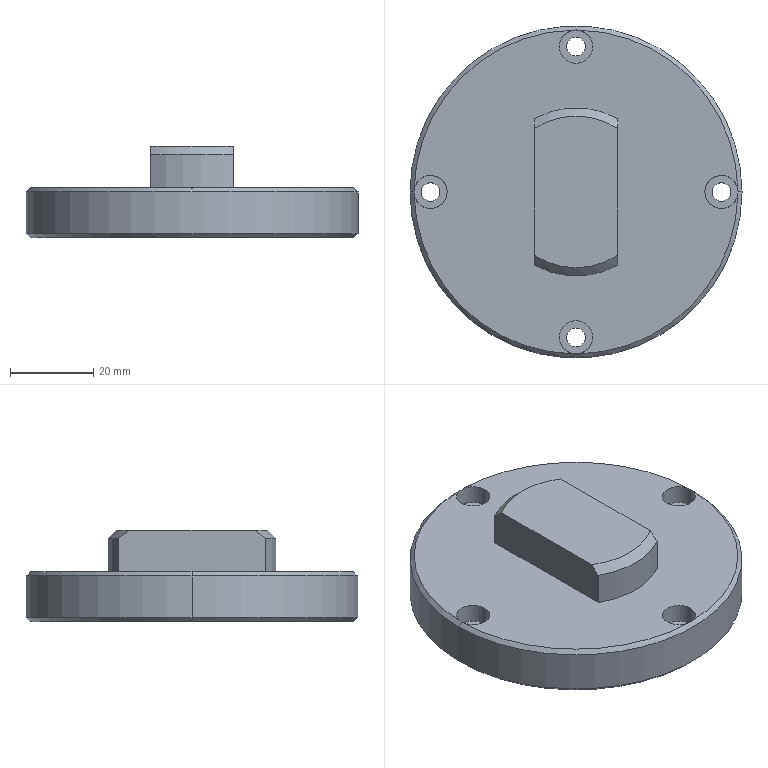Part | STEP file | TJ-DHQM-004-010 | 1 solid | 35 faces | box 79.9 x 79.9 x 22 mm | volume 66197 mm3 | cylinder 20 | plane 9 | cone 6 | commonest cylinder face diameters 4.5 x8 8 x8 40.5 x2 79.9 x2
STEP:
#1=CARTESIAN_POINT('',(-4.,35.,7.4));
#2=VERTEX_POINT('',#1);
#3=CARTESIAN_POINT('',(4.,35.,7.4));
#4=VERTEX_POINT('',#3);
#5=CARTESIAN_POINT('',(0.,35.,7.4));
#6=DIRECTION('',(0.,0.,1.));
#7=DIRECTION('',(1.,0.,0.));
#8=AXIS2_PLACEMENT_3D('',#5,#6,#7);
#9=CIRCLE('',#8,4.);
#10=EDGE_CURVE('',#2,#4,#9,.T.);
#11=ORIENTED_EDGE('',*,*,#10,.F.);
#12=CARTESIAN_POINT('',(-4.,35.,12.));
#13=VERTEX_POINT('',#12);
#14=CARTESIAN_POINT('',(-4.,35.,12.));
#15=DIRECTION('',(0.,0.,1.));
#16=VECTOR('',#15,1000.);
#17=LINE('',#14,#16);
#18=EDGE_CURVE('',#2,#13,#17,.T.);
#19=ORIENTED_EDGE('',*,*,#18,.T.);
#20=CARTESIAN_POINT('',(4.,35.,12.));
#21=VERTEX_POINT('',#20);
#22=CARTESIAN_POINT('',(0.,35.,12.));
#23=DIRECTION('',(0.,0.,1.));
#24=DIRECTION('',(1.,0.,0.));
#25=AXIS2_PLACEMENT_3D('',#22,#23,#24);
#26=CIRCLE('',#25,4.);
#27=EDGE_CURVE('',#13,#21,#26,.T.);
#28=ORIENTED_EDGE('',*,*,#27,.T.);
#29=CARTESIAN_POINT('',(4.,35.,12.));
#30=DIRECTION('',(0.,0.,1.));
#31=VECTOR('',#30,1000.);
#32=LINE('',#29,#31);
#33=EDGE_CURVE('',#4,#21,#32,.T.);
#34=ORIENTED_EDGE('',*,*,#33,.F.);
#35=EDGE_LOOP('',(#11,#19,#28,#34));
#36=FACE_OUTER_BOUND('',#35,.T.);
#37=CARTESIAN_POINT('',(0.,35.,12.));
#38=DIRECTION('',(0.,0.,1.));
#39=DIRECTION('',(1.,0.,0.));
#40=AXIS2_PLACEMENT_3D('',#37,#38,#39);
#41=CYLINDRICAL_SURFACE('',#40,4.);
#42=ADVANCED_FACE('',(#36),#41,.F.);
#43=CARTESIAN_POINT('',(-2.25,35.,0.));
#44=VERTEX_POINT('',#43);
#45=CARTESIAN_POINT('',(2.25,35.,0.));
#46=VERTEX_POINT('',#45);
#47=CARTESIAN_POINT('',(0.,35.,0.));
#48=DIRECTION('',(0.,0.,1.));
#49=DIRECTION('',(1.,0.,0.));
#50=AXIS2_PLACEMENT_3D('',#47,#48,#49);
#51=CIRCLE('',#50,2.25);
#52=EDGE_CURVE('',#44,#46,#51,.T.);
#53=ORIENTED_EDGE('',*,*,#52,.F.);
#54=CARTESIAN_POINT('',(-2.25,35.,7.4));
#55=VERTEX_POINT('',#54);
#56=CARTESIAN_POINT('',(-2.25,35.,12.));
#57=DIRECTION('',(0.,0.,1.));
#58=VECTOR('',#57,1000.);
#59=LINE('',#56,#58);
#60=EDGE_CURVE('',#44,#55,#59,.T.);
#61=ORIENTED_EDGE('',*,*,#60,.T.);
#62=CARTESIAN_POINT('',(2.25,35.,7.4));
#63=VERTEX_POINT('',#62);
#64=CARTESIAN_POINT('',(0.,35.,7.4));
#65=DIRECTION('',(0.,0.,1.));
#66=DIRECTION('',(1.,0.,0.));
#67=AXIS2_PLACEMENT_3D('',#64,#65,#66);
#68=CIRCLE('',#67,2.25);
#69=EDGE_CURVE('',#55,#63,#68,.T.);
#70=ORIENTED_EDGE('',*,*,#69,.T.);
#71=CARTESIAN_POINT('',(2.25,35.,12.));
#72=DIRECTION('',(0.,0.,1.));
#73=VECTOR('',#72,1000.);
#74=LINE('',#71,#73);
#75=EDGE_CURVE('',#46,#63,#74,.T.);
#76=ORIENTED_EDGE('',*,*,#75,.F.);
#77=EDGE_LOOP('',(#53,#61,#70,#76));
#78=FACE_OUTER_BOUND('',#77,.T.);
#79=CARTESIAN_POINT('',(0.,35.,12.));
#80=DIRECTION('',(0.,0.,1.));
#81=DIRECTION('',(1.,0.,0.));
#82=AXIS2_PLACEMENT_3D('',#79,#80,#81);
#83=CYLINDRICAL_SURFACE('',#82,2.25);
#84=ADVANCED_FACE('',(#78),#83,.F.);
#85=CARTESIAN_POINT('',(-39.,0.,7.4));
#86=VERTEX_POINT('',#85);
#87=CARTESIAN_POINT('',(-31.,0.,7.4));
#88=VERTEX_POINT('',#87);
#89=CARTESIAN_POINT('',(-35.,0.,7.4));
#90=DIRECTION('',(0.,0.,1.));
#91=DIRECTION('',(1.,0.,0.));
#92=AXIS2_PLACEMENT_3D('',#89,#90,#91);
#93=CIRCLE('',#92,4.);
#94=EDGE_CURVE('',#86,#88,#93,.T.);
#95=ORIENTED_EDGE('',*,*,#94,.F.);
#96=CARTESIAN_POINT('',(-39.,0.,11.95));
#97=VERTEX_POINT('',#96);
#98=CARTESIAN_POINT('',(-39.,0.,12.));
#99=DIRECTION('',(0.,0.,1.));
#100=VECTOR('',#99,1000.);
#101=LINE('',#98,#100);
#102=EDGE_CURVE('',#86,#97,#101,.T.);
#103=ORIENTED_EDGE('',*,*,#102,.T.);
#104=CARTESIAN_POINT('',(-38.944,-0.6651,12.));
#105=VERTEX_POINT('',#104);
#106=CARTESIAN_POINT('',(-39.,0.,11.95));
#107=CARTESIAN_POINT('',(-39.,-0.2216,11.95));
#108=CARTESIAN_POINT('',(-38.981,-0.4461,11.967));
#109=CARTESIAN_POINT('',(-38.944,-0.6651,12.));
#110=B_SPLINE_CURVE_WITH_KNOTS('',3,(#106,#107,#108,#109),.UNSPECIFIED.,.F.,.F.,(4,4),(0.0006695,0.001333),.UNSPECIFIED.);
#111=EDGE_CURVE('',#97,#105,#110,.T.);
#112=ORIENTED_EDGE('',*,*,#111,.T.);
#113=CARTESIAN_POINT('',(-31.,0.,12.));
#114=VERTEX_POINT('',#113);
#115=CARTESIAN_POINT('',(-35.,0.,12.));
#116=DIRECTION('',(0.,0.,1.));
#117=DIRECTION('',(1.,0.,0.));
#118=AXIS2_PLACEMENT_3D('',#115,#116,#117);
#119=CIRCLE('',#118,4.);
#120=EDGE_CURVE('',#105,#114,#119,.T.);
#121=ORIENTED_EDGE('',*,*,#120,.T.);
#122=CARTESIAN_POINT('',(-31.,0.,12.));
#123=DIRECTION('',(0.,0.,1.));
#124=VECTOR('',#123,1000.);
#125=LINE('',#122,#124);
#126=EDGE_CURVE('',#88,#114,#125,.T.);
#127=ORIENTED_EDGE('',*,*,#126,.F.);
#128=EDGE_LOOP('',(#95,#103,#112,#121,#127));
#129=FACE_OUTER_BOUND('',#128,.T.);
#130=CARTESIAN_POINT('',(-35.,0.,12.));
#131=DIRECTION('',(0.,0.,1.));
#132=DIRECTION('',(1.,0.,0.));
#133=AXIS2_PLACEMENT_3D('',#130,#131,#132);
#134=CYLINDRICAL_SURFACE('',#133,4.);
#135=ADVANCED_FACE('',(#129),#134,.F.);
#136=CARTESIAN_POINT('',(-37.25,0.,0.));
#137=VERTEX_POINT('',#136);
#138=CARTESIAN_POINT('',(-32.75,0.,0.));
#139=VERTEX_POINT('',#138);
#140=CARTESIAN_POINT('',(-35.,0.,0.));
#141=DIRECTION('',(0.,0.,1.));
#142=DIRECTION('',(1.,0.,0.));
#143=AXIS2_PLACEMENT_3D('',#140,#141,#142);
#144=CIRCLE('',#143,2.25);
#145=EDGE_CURVE('',#137,#139,#144,.T.);
#146=ORIENTED_EDGE('',*,*,#145,.F.);
#147=CARTESIAN_POINT('',(-37.25,0.,7.4));
#148=VERTEX_POINT('',#147);
#149=CARTESIAN_POINT('',(-37.25,0.,12.));
#150=DIRECTION('',(0.,0.,1.));
#151=VECTOR('',#150,1000.);
#152=LINE('',#149,#151);
#153=EDGE_CURVE('',#137,#148,#152,.T.);
#154=ORIENTED_EDGE('',*,*,#153,.T.);
#155=CARTESIAN_POINT('',(-32.75,0.,7.4));
#156=VERTEX_POINT('',#155);
#157=CARTESIAN_POINT('',(-35.,0.,7.4));
#158=DIRECTION('',(0.,0.,1.));
#159=DIRECTION('',(1.,0.,0.));
#160=AXIS2_PLACEMENT_3D('',#157,#158,#159);
#161=CIRCLE('',#160,2.25);
#162=EDGE_CURVE('',#148,#156,#161,.T.);
#163=ORIENTED_EDGE('',*,*,#162,.T.);
#164=CARTESIAN_POINT('',(-32.75,0.,12.));
#165=DIRECTION('',(0.,0.,1.));
#166=VECTOR('',#165,1000.);
#167=LINE('',#164,#166);
#168=EDGE_CURVE('',#139,#156,#167,.T.);
#169=ORIENTED_EDGE('',*,*,#168,.F.);
#170=EDGE_LOOP('',(#146,#154,#163,#169));
#171=FACE_OUTER_BOUND('',#170,.T.);
#172=CARTESIAN_POINT('',(-35.,0.,12.));
#173=DIRECTION('',(0.,0.,1.));
#174=DIRECTION('',(1.,0.,0.));
#175=AXIS2_PLACEMENT_3D('',#172,#173,#174);
#176=CYLINDRICAL_SURFACE('',#175,2.25);
#177=ADVANCED_FACE('',(#171),#176,.F.);
#178=CARTESIAN_POINT('',(-4.,-35.,7.4));
#179=VERTEX_POINT('',#178);
#180=CARTESIAN_POINT('',(4.,-35.,7.4));
#181=VERTEX_POINT('',#180);
#182=CARTESIAN_POINT('',(0.,-35.,7.4));
#183=DIRECTION('',(0.,0.,1.));
#184=DIRECTION('',(1.,0.,0.));
#185=AXIS2_PLACEMENT_3D('',#182,#183,#184);
#186=CIRCLE('',#185,4.);
#187=EDGE_CURVE('',#179,#181,#186,.T.);
#188=ORIENTED_EDGE('',*,*,#187,.F.);
#189=CARTESIAN_POINT('',(-4.,-35.,12.));
#190=VERTEX_POINT('',#189);
#191=CARTESIAN_POINT('',(-4.,-35.,12.));
#192=DIRECTION('',(0.,0.,1.));
#193=VECTOR('',#192,1000.);
#194=LINE('',#191,#193);
#195=EDGE_CURVE('',#179,#190,#194,.T.);
#196=ORIENTED_EDGE('',*,*,#195,.T.);
#197=CARTESIAN_POINT('',(-0.6651,-38.944,12.));
#198=VERTEX_POINT('',#197);
#199=CARTESIAN_POINT('',(0.,-35.,12.));
#200=DIRECTION('',(0.,0.,1.));
#201=DIRECTION('',(1.,0.,0.));
#202=AXIS2_PLACEMENT_3D('',#199,#200,#201);
#203=CIRCLE('',#202,4.);
#204=EDGE_CURVE('',#190,#198,#203,.T.);
#205=ORIENTED_EDGE('',*,*,#204,.T.);
#206=CARTESIAN_POINT('',(0.6651,-38.944,12.));
#207=VERTEX_POINT('',#206);
#208=CARTESIAN_POINT('',(-0.6651,-38.944,12.));
#209=CARTESIAN_POINT('',(-0.4455,-38.981,11.967));
#210=CARTESIAN_POINT('',(-0.2245,-39.,11.95));
#211=CARTESIAN_POINT('',(0.2202,-39.,11.95));
#212=CARTESIAN_POINT('',(0.4454,-38.981,11.967));
#213=CARTESIAN_POINT('',(0.6651,-38.944,12.));
#214=B_SPLINE_CURVE_WITH_KNOTS('',3,(#208,#209,#210,#211,#212,#213),.UNSPECIFIED.,.F.,.F.,(4,2,4),(0.000001333,0.0006674,0.001333),.UNSPECIFIED.);
#215=EDGE_CURVE('',#198,#207,#214,.T.);
#216=ORIENTED_EDGE('',*,*,#215,.T.);
#217=CARTESIAN_POINT('',(4.,-35.,12.));
#218=VERTEX_POINT('',#217);
#219=CARTESIAN_POINT('',(0.,-35.,12.));
#220=DIRECTION('',(0.,0.,1.));
#221=DIRECTION('',(1.,0.,0.));
#222=AXIS2_PLACEMENT_3D('',#219,#220,#221);
#223=CIRCLE('',#222,4.);
#224=EDGE_CURVE('',#207,#218,#223,.T.);
#225=ORIENTED_EDGE('',*,*,#224,.T.);
#226=CARTESIAN_POINT('',(4.,-35.,12.));
#227=DIRECTION('',(0.,0.,1.));
#228=VECTOR('',#227,1000.);
#229=LINE('',#226,#228);
#230=EDGE_CURVE('',#181,#218,#229,.T.);
#231=ORIENTED_EDGE('',*,*,#230,.F.);
#232=EDGE_LOOP('',(#188,#196,#205,#216,#225,#231));
#233=FACE_OUTER_BOUND('',#232,.T.);
#234=CARTESIAN_POINT('',(0.,-35.,12.));
#235=DIRECTION('',(0.,0.,1.));
#236=DIRECTION('',(1.,0.,0.));
#237=AXIS2_PLACEMENT_3D('',#234,#235,#236);
#238=CYLINDRICAL_SURFACE('',#237,4.);
#239=ADVANCED_FACE('',(#233),#238,.F.);
#240=CARTESIAN_POINT('',(-2.25,-35.,0.));
#241=VERTEX_POINT('',#240);
#242=CARTESIAN_POINT('',(2.25,-35.,0.));
#243=VERTEX_POINT('',#242);
#244=CARTESIAN_POINT('',(0.,-35.,0.));
#245=DIRECTION('',(0.,0.,1.));
#246=DIRECTION('',(1.,0.,0.));
#247=AXIS2_PLACEMENT_3D('',#244,#245,#246);
#248=CIRCLE('',#247,2.25);
#249=EDGE_CURVE('',#241,#243,#248,.T.);
#250=ORIENTED_EDGE('',*,*,#249,.F.);
#251=CARTESIAN_POINT('',(-2.25,-35.,7.4));
#252=VERTEX_POINT('',#251);
#253=CARTESIAN_POINT('',(-2.25,-35.,12.));
#254=DIRECTION('',(0.,0.,1.));
#255=VECTOR('',#254,1000.);
#256=LINE('',#253,#255);
#257=EDGE_CURVE('',#241,#252,#256,.T.);
#258=ORIENTED_EDGE('',*,*,#257,.T.);
#259=CARTESIAN_POINT('',(2.25,-35.,7.4));
#260=VERTEX_POINT('',#259);
#261=CARTESIAN_POINT('',(0.,-35.,7.4));
#262=DIRECTION('',(0.,0.,1.));
#263=DIRECTION('',(1.,0.,0.));
#264=AXIS2_PLACEMENT_3D('',#261,#262,#263);
#265=CIRCLE('',#264,2.25);
#266=EDGE_CURVE('',#252,#260,#265,.T.);
#267=ORIENTED_EDGE('',*,*,#266,.T.);
#268=CARTESIAN_POINT('',(2.25,-35.,12.));
#269=DIRECTION('',(0.,0.,1.));
#270=VECTOR('',#269,1000.);
#271=LINE('',#268,#270);
#272=EDGE_CURVE('',#243,#260,#271,.T.);
#273=ORIENTED_EDGE('',*,*,#272,.F.);
#274=EDGE_LOOP('',(#250,#258,#267,#273));
#275=FACE_OUTER_BOUND('',#274,.T.);
#276=CARTESIAN_POINT('',(0.,-35.,12.));
#277=DIRECTION('',(0.,0.,1.));
#278=DIRECTION('',(1.,0.,0.));
#279=AXIS2_PLACEMENT_3D('',#276,#277,#278);
#280=CYLINDRICAL_SURFACE('',#279,2.25);
#281=ADVANCED_FACE('',(#275),#280,.F.);
#282=CARTESIAN_POINT('',(31.,0.,7.4));
#283=VERTEX_POINT('',#282);
#284=CARTESIAN_POINT('',(39.,0.,7.4));
#285=VERTEX_POINT('',#284);
#286=CARTESIAN_POINT('',(35.,0.,7.4));
#287=DIRECTION('',(0.,0.,1.));
#288=DIRECTION('',(1.,0.,0.));
#289=AXIS2_PLACEMENT_3D('',#286,#287,#288);
#290=CIRCLE('',#289,4.);
#291=EDGE_CURVE('',#283,#285,#290,.T.);
#292=ORIENTED_EDGE('',*,*,#291,.F.);
#293=CARTESIAN_POINT('',(31.,0.,12.));
#294=VERTEX_POINT('',#293);
#295=CARTESIAN_POINT('',(31.,0.,12.));
#296=DIRECTION('',(0.,0.,1.));
#297=VECTOR('',#296,1000.);
#298=LINE('',#295,#297);
#299=EDGE_CURVE('',#283,#294,#298,.T.);
#300=ORIENTED_EDGE('',*,*,#299,.T.);
#301=CARTESIAN_POINT('',(38.944,-0.6651,12.));
#302=VERTEX_POINT('',#301);
#303=CARTESIAN_POINT('',(35.,0.,12.));
#304=DIRECTION('',(0.,0.,1.));
#305=DIRECTION('',(1.,0.,0.));
#306=AXIS2_PLACEMENT_3D('',#303,#304,#305);
#307=CIRCLE('',#306,4.);
#308=EDGE_CURVE('',#294,#302,#307,.T.);
#309=ORIENTED_EDGE('',*,*,#308,.T.);
#310=CARTESIAN_POINT('',(39.,0.,11.95));
#311=VERTEX_POINT('',#310);
#312=CARTESIAN_POINT('',(38.944,-0.6651,12.));
#313=CARTESIAN_POINT('',(38.981,-0.4448,11.967));
#314=CARTESIAN_POINT('',(39.,-0.2231,11.95));
#315=CARTESIAN_POINT('',(39.,0.,11.95));
#316=B_SPLINE_CURVE_WITH_KNOTS('',3,(#312,#313,#314,#315),.UNSPECIFIED.,.F.,.F.,(4,4),(0.000001333,0.0006695),.UNSPECIFIED.);
#317=EDGE_CURVE('',#302,#311,#316,.T.);
#318=ORIENTED_EDGE('',*,*,#317,.T.);
#319=CARTESIAN_POINT('',(39.,0.,12.));
#320=DIRECTION('',(0.,0.,1.));
#321=VECTOR('',#320,1000.);
#322=LINE('',#319,#321);
#323=EDGE_CURVE('',#285,#311,#322,.T.);
#324=ORIENTED_EDGE('',*,*,#323,.F.);
#325=EDGE_LOOP('',(#292,#300,#309,#318,#324));
#326=FACE_OUTER_BOUND('',#325,.T.);
#327=CARTESIAN_POINT('',(35.,0.,12.));
#328=DIRECTION('',(0.,0.,1.));
#329=DIRECTION('',(1.,0.,0.));
#330=AXIS2_PLACEMENT_3D('',#327,#328,#329);
#331=CYLINDRICAL_SURFACE('',#330,4.);
#332=ADVANCED_FACE('',(#326),#331,.F.);
#333=CARTESIAN_POINT('',(32.75,0.,0.));
#334=VERTEX_POINT('',#333);
#335=CARTESIAN_POINT('',(37.25,0.,0.));
#336=VERTEX_POINT('',#335);
#337=CARTESIAN_POINT('',(35.,0.,0.));
#338=DIRECTION('',(0.,0.,1.));
#339=DIRECTION('',(1.,0.,0.));
#340=AXIS2_PLACEMENT_3D('',#337,#338,#339);
#341=CIRCLE('',#340,2.25);
#342=EDGE_CURVE('',#334,#336,#341,.T.);
#343=ORIENTED_EDGE('',*,*,#342,.F.);
#344=CARTESIAN_POINT('',(32.75,0.,7.4));
#345=VERTEX_POINT('',#344);
#346=CARTESIAN_POINT('',(32.75,0.,12.));
#347=DIRECTION('',(0.,0.,1.));
#348=VECTOR('',#347,1000.);
#349=LINE('',#346,#348);
#350=EDGE_CURVE('',#334,#345,#349,.T.);
#351=ORIENTED_EDGE('',*,*,#350,.T.);
#352=CARTESIAN_POINT('',(37.25,0.,7.4));
#353=VERTEX_POINT('',#352);
#354=CARTESIAN_POINT('',(35.,0.,7.4));
#355=DIRECTION('',(0.,0.,1.));
#356=DIRECTION('',(1.,0.,0.));
#357=AXIS2_PLACEMENT_3D('',#354,#355,#356);
#358=CIRCLE('',#357,2.25);
#359=EDGE_CURVE('',#345,#353,#358,.T.);
#360=ORIENTED_EDGE('',*,*,#359,.T.);
#361=CARTESIAN_POINT('',(37.25,0.,12.));
#362=DIRECTION('',(0.,0.,1.));
#363=VECTOR('',#362,1000.);
#364=LINE('',#361,#363);
#365=EDGE_CURVE('',#336,#353,#364,.T.);
#366=ORIENTED_EDGE('',*,*,#365,.F.);
#367=EDGE_LOOP('',(#343,#351,#360,#366));
#368=FACE_OUTER_BOUND('',#367,.T.);
#369=CARTESIAN_POINT('',(35.,0.,12.));
#370=DIRECTION('',(0.,0.,1.));
#371=DIRECTION('',(1.,0.,0.));
#372=AXIS2_PLACEMENT_3D('',#369,#370,#371);
#373=CYLINDRICAL_SURFACE('',#372,2.25);
#374=ADVANCED_FACE('',(#368),#373,.F.);
#375=CARTESIAN_POINT('',(38.944,0.6651,12.));
#376=VERTEX_POINT('',#375);
#377=CARTESIAN_POINT('',(39.,0.,11.95));
#378=CARTESIAN_POINT('',(39.,0.2216,11.95));
#379=CARTESIAN_POINT('',(38.981,0.4461,11.967));
#380=CARTESIAN_POINT('',(38.944,0.6651,12.));
#381=B_SPLINE_CURVE_WITH_KNOTS('',3,(#377,#378,#379,#380),.UNSPECIFIED.,.F.,.F.,(4,4),(0.0006695,0.001333),.UNSPECIFIED.);
#382=EDGE_CURVE('',#311,#376,#381,.T.);
#383=ORIENTED_EDGE('',*,*,#382,.F.);
#384=CARTESIAN_POINT('',(39.95,0.,11.));
#385=VERTEX_POINT('',#384);
#386=CARTESIAN_POINT('',(38.95,0.,12.));
#387=DIRECTION('',(0.7071,0.,-0.7071));
#388=VECTOR('',#387,1000.);
#389=LINE('',#386,#388);
#390=EDGE_CURVE('',#311,#385,#389,.T.);
#391=ORIENTED_EDGE('',*,*,#390,.T.);
#392=CARTESIAN_POINT('',(-39.95,0.,11.));
#393=VERTEX_POINT('',#392);
#394=CARTESIAN_POINT('',(0.,0.,11.));
#395=DIRECTION('',(0.,0.,-1.));
#396=DIRECTION('',(1.,0.,0.));
#397=AXIS2_PLACEMENT_3D('',#394,#395,#396);
#398=CIRCLE('',#397,39.95);
#399=EDGE_CURVE('',#393,#385,#398,.T.);
#400=ORIENTED_EDGE('',*,*,#399,.F.);
#401=CARTESIAN_POINT('',(-38.95,0.,12.));
#402=DIRECTION('',(-0.7071,0.,-0.7071));
#403=VECTOR('',#402,1000.);
#404=LINE('',#401,#403);
#405=EDGE_CURVE('',#97,#393,#404,.T.);
#406=ORIENTED_EDGE('',*,*,#405,.F.);
#407=CARTESIAN_POINT('',(-38.944,0.6651,12.));
#408=VERTEX_POINT('',#407);
#409=CARTESIAN_POINT('',(-38.944,0.6651,12.));
#410=CARTESIAN_POINT('',(-38.981,0.4448,11.967));
#411=CARTESIAN_POINT('',(-39.,0.2231,11.95));
#412=CARTESIAN_POINT('',(-39.,0.,11.95));
#413=B_SPLINE_CURVE_WITH_KNOTS('',3,(#409,#410,#411,#412),.UNSPECIFIED.,.F.,.F.,(4,4),(0.000001333,0.0006695),.UNSPECIFIED.);
#414=EDGE_CURVE('',#408,#97,#413,.T.);
#415=ORIENTED_EDGE('',*,*,#414,.F.);
#416=CARTESIAN_POINT('',(-0.6651,38.944,12.));
#417=VERTEX_POINT('',#416);
#418=CARTESIAN_POINT('',(0.,0.,12.));
#419=DIRECTION('',(0.,0.,1.));
#420=DIRECTION('',(1.,0.,0.));
#421=AXIS2_PLACEMENT_3D('',#418,#419,#420);
#422=CIRCLE('',#421,38.95);
#423=EDGE_CURVE('',#417,#408,#422,.T.);
#424=ORIENTED_EDGE('',*,*,#423,.F.);
#425=CARTESIAN_POINT('',(0.6651,38.944,12.));
#426=VERTEX_POINT('',#425);
#427=CARTESIAN_POINT('',(0.6651,38.944,12.));
#428=CARTESIAN_POINT('',(0.4455,38.981,11.967));
#429=CARTESIAN_POINT('',(0.2245,39.,11.95));
#430=CARTESIAN_POINT('',(-0.2202,39.,11.95));
#431=CARTESIAN_POINT('',(-0.4454,38.981,11.967));
#432=CARTESIAN_POINT('',(-0.6651,38.944,12.));
#433=B_SPLINE_CURVE_WITH_KNOTS('',3,(#427,#428,#429,#430,#431,#432),.UNSPECIFIED.,.F.,.F.,(4,2,4),(0.000001333,0.0006674,0.001333),.UNSPECIFIED.);
#434=EDGE_CURVE('',#426,#417,#433,.T.);
#435=ORIENTED_EDGE('',*,*,#434,.F.);
#436=CARTESIAN_POINT('',(0.,0.,12.));
#437=DIRECTION('',(0.,0.,1.));
#438=DIRECTION('',(1.,0.,0.));
#439=AXIS2_PLACEMENT_3D('',#436,#437,#438);
#440=CIRCLE('',#439,38.95);
#441=EDGE_CURVE('',#376,#426,#440,.T.);
#442=ORIENTED_EDGE('',*,*,#441,.F.);
#443=EDGE_LOOP('',(#383,#391,#400,#406,#415,#424,#435,#442));
#444=FACE_OUTER_BOUND('',#443,.T.);
#445=CARTESIAN_POINT('',(0.,0.,12.));
#446=DIRECTION('',(0.,0.,-1.));
#447=DIRECTION('',(-1.,0.,0.));
#448=AXIS2_PLACEMENT_3D('',#445,#446,#447);
#449=CONICAL_SURFACE('',#448,38.95,0.7854);
#450=ADVANCED_FACE('',(#444),#449,.T.);
#451=CARTESIAN_POINT('',(-38.95,0.,0.));
#452=VERTEX_POINT('',#451);
#453=CARTESIAN_POINT('',(38.95,0.,0.));
#454=VERTEX_POINT('',#453);
#455=CARTESIAN_POINT('',(0.,0.,0.));
#456=DIRECTION('',(0.,0.,-1.));
#457=DIRECTION('',(1.,0.,0.));
#458=AXIS2_PLACEMENT_3D('',#455,#456,#457);
#459=CIRCLE('',#458,38.95);
#460=EDGE_CURVE('',#452,#454,#459,.T.);
#461=ORIENTED_EDGE('',*,*,#460,.F.);
#462=CARTESIAN_POINT('',(-39.95,0.,1.));
#463=VERTEX_POINT('',#462);
#464=CARTESIAN_POINT('',(-39.95,0.,1.));
#465=DIRECTION('',(-0.7071,0.,0.7071));
#466=VECTOR('',#465,1000.);
#467=LINE('',#464,#466);
#468=EDGE_CURVE('',#452,#463,#467,.T.);
#469=ORIENTED_EDGE('',*,*,#468,.T.);
#470=CARTESIAN_POINT('',(39.95,0.,1.));
#471=VERTEX_POINT('',#470);
#472=CARTESIAN_POINT('',(0.,0.,1.));
#473=DIRECTION('',(0.,0.,1.));
#474=DIRECTION('',(1.,0.,0.));
#475=AXIS2_PLACEMENT_3D('',#472,#473,#474);
#476=CIRCLE('',#475,39.95);
#477=EDGE_CURVE('',#471,#463,#476,.T.);
#478=ORIENTED_EDGE('',*,*,#477,.F.);
#479=CARTESIAN_POINT('',(39.95,0.,1.));
#480=DIRECTION('',(0.7071,0.,0.7071));
#481=VECTOR('',#480,1000.);
#482=LINE('',#479,#481);
#483=EDGE_CURVE('',#454,#471,#482,.T.);
#484=ORIENTED_EDGE('',*,*,#483,.F.);
#485=EDGE_LOOP('',(#461,#469,#478,#484));
#486=FACE_OUTER_BOUND('',#485,.T.);
#487=CARTESIAN_POINT('',(0.,0.,1.));
#488=DIRECTION('',(0.,0.,1.));
#489=DIRECTION('',(1.,0.,0.));
#490=AXIS2_PLACEMENT_3D('',#487,#488,#489);
#491=CONICAL_SURFACE('',#490,39.95,0.7854);
#492=ADVANCED_FACE('',(#486),#491,.T.);
#493=ORIENTED_EDGE('',*,*,#399,.T.);
#494=CARTESIAN_POINT('',(39.95,0.,12.));
#495=DIRECTION('',(0.,0.,-1.));
#496=VECTOR('',#495,1000.);
#497=LINE('',#494,#496);
#498=EDGE_CURVE('',#385,#471,#497,.T.);
#499=ORIENTED_EDGE('',*,*,#498,.T.);
#500=ORIENTED_EDGE('',*,*,#477,.T.);
#501=CARTESIAN_POINT('',(-39.95,0.,12.));
#502=DIRECTION('',(0.,0.,-1.));
#503=VECTOR('',#502,1000.);
#504=LINE('',#501,#503);
#505=EDGE_CURVE('',#393,#463,#504,.T.);
#506=ORIENTED_EDGE('',*,*,#505,.F.);
#507=EDGE_LOOP('',(#493,#499,#500,#506));
#508=FACE_OUTER_BOUND('',#507,.T.);
#509=CARTESIAN_POINT('',(0.,0.,12.));
#510=DIRECTION('',(0.,0.,-1.));
#511=DIRECTION('',(-1.,0.,0.));
#512=AXIS2_PLACEMENT_3D('',#509,#510,#511);
#513=CYLINDRICAL_SURFACE('',#512,39.95);
#514=ADVANCED_FACE('',(#508),#513,.T.);
#515=CARTESIAN_POINT('',(10.,-17.609,20.));
#516=VERTEX_POINT('',#515);
#517=CARTESIAN_POINT('',(-10.,-17.609,20.));
#518=VERTEX_POINT('',#517);
#519=CARTESIAN_POINT('',(0.,0.,20.));
#520=DIRECTION('',(0.,0.,-1.));
#521=DIRECTION('',(1.,0.,0.));
#522=AXIS2_PLACEMENT_3D('',#519,#520,#521);
#523=CIRCLE('',#522,20.25);
#524=EDGE_CURVE('',#516,#518,#523,.T.);
#525=ORIENTED_EDGE('',*,*,#524,.T.);
#526=CARTESIAN_POINT('',(-10.,-17.609,12.));
#527=VERTEX_POINT('',#526);
#528=CARTESIAN_POINT('',(-10.,-17.609,22.));
#529=DIRECTION('',(0.,0.,-1.));
#530=VECTOR('',#529,1000.);
#531=LINE('',#528,#530);
#532=EDGE_CURVE('',#518,#527,#531,.T.);
#533=ORIENTED_EDGE('',*,*,#532,.T.);
#534=CARTESIAN_POINT('',(10.,-17.609,12.));
#535=VERTEX_POINT('',#534);
#536=CARTESIAN_POINT('',(0.,0.,12.));
#537=DIRECTION('',(0.,0.,1.));
#538=DIRECTION('',(1.,0.,0.));
#539=AXIS2_PLACEMENT_3D('',#536,#537,#538);
#540=CIRCLE('',#539,20.25);
#541=EDGE_CURVE('',#527,#535,#540,.T.);
#542=ORIENTED_EDGE('',*,*,#541,.T.);
#543=CARTESIAN_POINT('',(10.,-17.609,22.));
#544=DIRECTION('',(0.,0.,1.));
#545=VECTOR('',#544,1000.);
#546=LINE('',#543,#545);
#547=EDGE_CURVE('',#535,#516,#546,.T.);
#548=ORIENTED_EDGE('',*,*,#547,.T.);
#549=EDGE_LOOP('',(#525,#533,#542,#548));
#550=FACE_OUTER_BOUND('',#549,.T.);
#551=CARTESIAN_POINT('',(0.,0.,22.));
#552=DIRECTION('',(0.,0.,-1.));
#553=DIRECTION('',(-1.,0.,0.));
#554=AXIS2_PLACEMENT_3D('',#551,#552,#553);
#555=CYLINDRICAL_SURFACE('',#554,20.25);
#556=ADVANCED_FACE('',(#550),#555,.T.);
#557=CARTESIAN_POINT('',(-10.,-15.266,22.));
#558=VERTEX_POINT('',#557);
#559=CARTESIAN_POINT('',(-10.,-17.609,20.));
#560=CARTESIAN_POINT('',(-10.,-16.834,20.674));
#561=CARTESIAN_POINT('',(-10.,-16.054,21.341));
#562=CARTESIAN_POINT('',(-10.,-15.266,22.));
#563=B_SPLINE_CURVE_WITH_KNOTS('',3,(#559,#560,#561,#562),.UNSPECIFIED.,.F.,.F.,(4,4),(0.000001066,0.00308),.UNSPECIFIED.);
#564=EDGE_CURVE('',#518,#558,#563,.T.);
#565=ORIENTED_EDGE('',*,*,#564,.F.);
#566=ORIENTED_EDGE('',*,*,#524,.F.);
#567=CARTESIAN_POINT('',(10.,-15.266,22.));
#568=VERTEX_POINT('',#567);
#569=CARTESIAN_POINT('',(10.,-15.266,22.));
#570=CARTESIAN_POINT('',(10.,-16.054,21.341));
#571=CARTESIAN_POINT('',(10.,-16.834,20.674));
#572=CARTESIAN_POINT('',(10.,-17.609,20.));
#573=B_SPLINE_CURVE_WITH_KNOTS('',3,(#569,#570,#571,#572),.UNSPECIFIED.,.F.,.F.,(4,4),(0.03846,0.04155),.UNSPECIFIED.);
#574=EDGE_CURVE('',#568,#516,#573,.T.);
#575=ORIENTED_EDGE('',*,*,#574,.F.);
#576=CARTESIAN_POINT('',(0.,0.,22.));
#577=DIRECTION('',(0.,0.,1.));
#578=DIRECTION('',(1.,0.,0.));
#579=AXIS2_PLACEMENT_3D('',#576,#577,#578);
#580=CIRCLE('',#579,18.25);
#581=EDGE_CURVE('',#558,#568,#580,.T.);
#582=ORIENTED_EDGE('',*,*,#581,.F.);
#583=EDGE_LOOP('',(#565,#566,#575,#582));
#584=FACE_OUTER_BOUND('',#583,.T.);
#585=CARTESIAN_POINT('',(0.,0.,22.));
#586=DIRECTION('',(0.,0.,-1.));
#587=DIRECTION('',(-1.,0.,0.));
#588=AXIS2_PLACEMENT_3D('',#585,#586,#587);
#589=CONICAL_SURFACE('',#588,18.25,0.7854);
#590=ADVANCED_FACE('',(#584),#589,.T.);
#591=ORIENTED_EDGE('',*,*,#498,.F.);
#592=CARTESIAN_POINT('',(0.,0.,11.));
#593=DIRECTION('',(0.,0.,-1.));
#594=DIRECTION('',(1.,0.,0.));
#595=AXIS2_PLACEMENT_3D('',#592,#593,#594);
#596=CIRCLE('',#595,39.95);
#597=EDGE_CURVE('',#385,#393,#596,.T.);
#598=ORIENTED_EDGE('',*,*,#597,.T.);
#599=ORIENTED_EDGE('',*,*,#505,.T.);
#600=CARTESIAN_POINT('',(0.,0.,1.));
#601=DIRECTION('',(0.,0.,1.));
#602=DIRECTION('',(1.,0.,0.));
#603=AXIS2_PLACEMENT_3D('',#600,#601,#602);
#604=CIRCLE('',#603,39.95);
#605=EDGE_CURVE('',#463,#471,#604,.T.);
#606=ORIENTED_EDGE('',*,*,#605,.T.);
#607=EDGE_LOOP('',(#591,#598,#599,#606));
#608=FACE_OUTER_BOUND('',#607,.T.);
#609=CARTESIAN_POINT('',(0.,0.,12.));
#610=DIRECTION('',(0.,0.,-1.));
#611=DIRECTION('',(-1.,0.,0.));
#612=AXIS2_PLACEMENT_3D('',#609,#610,#611);
#613=CYLINDRICAL_SURFACE('',#612,39.95);
#614=ADVANCED_FACE('',(#608),#613,.T.);
#615=ORIENTED_EDGE('',*,*,#541,.F.);
#616=CARTESIAN_POINT('',(-10.,17.609,12.));
#617=VERTEX_POINT('',#616);
#618=CARTESIAN_POINT('',(-10.,22.18,12.));
#619=DIRECTION('',(0.,1.,0.));
#620=VECTOR('',#619,1000.);
#621=LINE('',#618,#620);
#622=EDGE_CURVE('',#527,#617,#621,.T.);
#623=ORIENTED_EDGE('',*,*,#622,.T.);
#624=CARTESIAN_POINT('',(10.,17.609,12.));
#625=VERTEX_POINT('',#624);
#626=CARTESIAN_POINT('',(0.,0.,12.));
#627=DIRECTION('',(0.,0.,1.));
#628=DIRECTION('',(1.,0.,0.));
#629=AXIS2_PLACEMENT_3D('',#626,#627,#628);
#630=CIRCLE('',#629,20.25);
#631=EDGE_CURVE('',#625,#617,#630,.T.);
#632=ORIENTED_EDGE('',*,*,#631,.F.);
#633=CARTESIAN_POINT('',(10.,22.18,12.));
#634=DIRECTION('',(0.,-1.,0.));
#635=VECTOR('',#634,1000.);
#636=LINE('',#633,#635);
#637=EDGE_CURVE('',#625,#535,#636,.T.);
#638=ORIENTED_EDGE('',*,*,#637,.T.);
#639=EDGE_LOOP('',(#615,#623,#632,#638));
#640=FACE_BOUND('',#639,.T.);
#641=CARTESIAN_POINT('',(0.,35.,12.));
#642=DIRECTION('',(0.,0.,1.));
#643=DIRECTION('',(1.,0.,0.));
#644=AXIS2_PLACEMENT_3D('',#641,#642,#643);
#645=CIRCLE('',#644,4.);
#646=EDGE_CURVE('',#417,#13,#645,.T.);
#647=ORIENTED_EDGE('',*,*,#646,.F.);
#648=ORIENTED_EDGE('',*,*,#423,.T.);
#649=CARTESIAN_POINT('',(-35.,0.,12.));
#650=DIRECTION('',(0.,0.,1.));
#651=DIRECTION('',(1.,0.,0.));
#652=AXIS2_PLACEMENT_3D('',#649,#650,#651);
#653=CIRCLE('',#652,4.);
#654=EDGE_CURVE('',#114,#408,#653,.T.);
#655=ORIENTED_EDGE('',*,*,#654,.F.);
#656=ORIENTED_EDGE('',*,*,#120,.F.);
#657=CARTESIAN_POINT('',(0.,0.,12.));
#658=DIRECTION('',(0.,0.,1.));
#659=DIRECTION('',(1.,0.,0.));
#660=AXIS2_PLACEMENT_3D('',#657,#658,#659);
#661=CIRCLE('',#660,38.95);
#662=EDGE_CURVE('',#105,#198,#661,.T.);
#663=ORIENTED_EDGE('',*,*,#662,.T.);
#664=ORIENTED_EDGE('',*,*,#204,.F.);
#665=CARTESIAN_POINT('',(0.,-35.,12.));
#666=DIRECTION('',(0.,0.,1.));
#667=DIRECTION('',(1.,0.,0.));
#668=AXIS2_PLACEMENT_3D('',#665,#666,#667);
#669=CIRCLE('',#668,4.);
#670=EDGE_CURVE('',#218,#190,#669,.T.);
#671=ORIENTED_EDGE('',*,*,#670,.F.);
#672=ORIENTED_EDGE('',*,*,#224,.F.);
#673=CARTESIAN_POINT('',(0.,0.,12.));
#674=DIRECTION('',(0.,0.,1.));
#675=DIRECTION('',(1.,0.,0.));
#676=AXIS2_PLACEMENT_3D('',#673,#674,#675);
#677=CIRCLE('',#676,38.95);
#678=EDGE_CURVE('',#207,#302,#677,.T.);
#679=ORIENTED_EDGE('',*,*,#678,.T.);
#680=ORIENTED_EDGE('',*,*,#308,.F.);
#681=CARTESIAN_POINT('',(35.,0.,12.));
#682=DIRECTION('',(0.,0.,1.));
#683=DIRECTION('',(1.,0.,0.));
#684=AXIS2_PLACEMENT_3D('',#681,#682,#683);
#685=CIRCLE('',#684,4.);
#686=EDGE_CURVE('',#376,#294,#685,.T.);
#687=ORIENTED_EDGE('',*,*,#686,.F.);
#688=ORIENTED_EDGE('',*,*,#441,.T.);
#689=CARTESIAN_POINT('',(0.,35.,12.));
#690=DIRECTION('',(0.,0.,1.));
#691=DIRECTION('',(1.,0.,0.));
#692=AXIS2_PLACEMENT_3D('',#689,#690,#691);
#693=CIRCLE('',#692,4.);
#694=EDGE_CURVE('',#21,#426,#693,.T.);
#695=ORIENTED_EDGE('',*,*,#694,.F.);
#696=ORIENTED_EDGE('',*,*,#27,.F.);
#697=EDGE_LOOP('',(#647,#648,#655,#656,#663,#664,#671,#672,#679,#680,#687,#688,#695,#696));
#698=FACE_OUTER_BOUND('',#697,.T.);
#699=CARTESIAN_POINT('',(0.,0.,12.));
#700=DIRECTION('',(0.,0.,1.));
#701=DIRECTION('',(1.,0.,0.));
#702=AXIS2_PLACEMENT_3D('',#699,#700,#701);
#703=PLANE('',#702);
#704=ADVANCED_FACE('',(#640,#698),#703,.T.);
#705=CARTESIAN_POINT('',(0.,35.,0.));
#706=DIRECTION('',(0.,0.,1.));
#707=DIRECTION('',(1.,0.,0.));
#708=AXIS2_PLACEMENT_3D('',#705,#706,#707);
#709=CIRCLE('',#708,2.25);
#710=EDGE_CURVE('',#46,#44,#709,.T.);
#711=ORIENTED_EDGE('',*,*,#710,.T.);
#712=ORIENTED_EDGE('',*,*,#52,.T.);
#713=EDGE_LOOP('',(#711,#712));
#714=FACE_BOUND('',#713,.T.);
#715=CARTESIAN_POINT('',(-35.,0.,0.));
#716=DIRECTION('',(0.,0.,1.));
#717=DIRECTION('',(1.,0.,0.));
#718=AXIS2_PLACEMENT_3D('',#715,#716,#717);
#719=CIRCLE('',#718,2.25);
#720=EDGE_CURVE('',#139,#137,#719,.T.);
#721=ORIENTED_EDGE('',*,*,#720,.T.);
#722=ORIENTED_EDGE('',*,*,#145,.T.);
#723=EDGE_LOOP('',(#721,#722));
#724=FACE_BOUND('',#723,.T.);
#725=CARTESIAN_POINT('',(0.,-35.,0.));
#726=DIRECTION('',(0.,0.,1.));
#727=DIRECTION('',(1.,0.,0.));
#728=AXIS2_PLACEMENT_3D('',#725,#726,#727);
#729=CIRCLE('',#728,2.25);
#730=EDGE_CURVE('',#243,#241,#729,.T.);
#731=ORIENTED_EDGE('',*,*,#730,.T.);
#732=ORIENTED_EDGE('',*,*,#249,.T.);
#733=EDGE_LOOP('',(#731,#732));
#734=FACE_BOUND('',#733,.T.);
#735=CARTESIAN_POINT('',(35.,0.,0.));
#736=DIRECTION('',(0.,0.,1.));
#737=DIRECTION('',(1.,0.,0.));
#738=AXIS2_PLACEMENT_3D('',#735,#736,#737);
#739=CIRCLE('',#738,2.25);
#740=EDGE_CURVE('',#336,#334,#739,.T.);
#741=ORIENTED_EDGE('',*,*,#740,.T.);
#742=ORIENTED_EDGE('',*,*,#342,.T.);
#743=EDGE_LOOP('',(#741,#742));
#744=FACE_BOUND('',#743,.T.);
#745=CARTESIAN_POINT('',(0.,0.,0.));
#746=DIRECTION('',(0.,0.,-1.));
#747=DIRECTION('',(1.,0.,0.));
#748=AXIS2_PLACEMENT_3D('',#745,#746,#747);
#749=CIRCLE('',#748,38.95);
#750=EDGE_CURVE('',#454,#452,#749,.T.);
#751=ORIENTED_EDGE('',*,*,#750,.T.);
#752=ORIENTED_EDGE('',*,*,#460,.T.);
#753=EDGE_LOOP('',(#751,#752));
#754=FACE_OUTER_BOUND('',#753,.T.);
#755=CARTESIAN_POINT('',(0.,0.,0.));
#756=DIRECTION('',(0.,0.,1.));
#757=DIRECTION('',(1.,0.,0.));
#758=AXIS2_PLACEMENT_3D('',#755,#756,#757);
#759=PLANE('',#758);
#760=ADVANCED_FACE('',(#714,#724,#734,#744,#754),#759,.F.);
#761=ORIENTED_EDGE('',*,*,#468,.F.);
#762=ORIENTED_EDGE('',*,*,#750,.F.);
#763=ORIENTED_EDGE('',*,*,#483,.T.);
#764=ORIENTED_EDGE('',*,*,#605,.F.);
#765=EDGE_LOOP('',(#761,#762,#763,#764));
#766=FACE_OUTER_BOUND('',#765,.T.);
#767=CARTESIAN_POINT('',(0.,0.,1.));
#768=DIRECTION('',(0.,0.,1.));
#769=DIRECTION('',(1.,0.,0.));
#770=AXIS2_PLACEMENT_3D('',#767,#768,#769);
#771=CONICAL_SURFACE('',#770,39.95,0.7854);
#772=ADVANCED_FACE('',(#766),#771,.T.);
#773=ORIENTED_EDGE('',*,*,#390,.F.);
#774=ORIENTED_EDGE('',*,*,#317,.F.);
#775=ORIENTED_EDGE('',*,*,#678,.F.);
#776=ORIENTED_EDGE('',*,*,#215,.F.);
#777=ORIENTED_EDGE('',*,*,#662,.F.);
#778=ORIENTED_EDGE('',*,*,#111,.F.);
#779=ORIENTED_EDGE('',*,*,#405,.T.);
#780=ORIENTED_EDGE('',*,*,#597,.F.);
#781=EDGE_LOOP('',(#773,#774,#775,#776,#777,#778,#779,#780));
#782=FACE_OUTER_BOUND('',#781,.T.);
#783=CARTESIAN_POINT('',(0.,0.,12.));
#784=DIRECTION('',(0.,0.,-1.));
#785=DIRECTION('',(-1.,0.,0.));
#786=AXIS2_PLACEMENT_3D('',#783,#784,#785);
#787=CONICAL_SURFACE('',#786,38.95,0.7854);
#788=ADVANCED_FACE('',(#782),#787,.T.);
#789=ORIENTED_EDGE('',*,*,#350,.F.);
#790=ORIENTED_EDGE('',*,*,#740,.F.);
#791=ORIENTED_EDGE('',*,*,#365,.T.);
#792=CARTESIAN_POINT('',(35.,0.,7.4));
#793=DIRECTION('',(0.,0.,1.));
#794=DIRECTION('',(1.,0.,0.));
#795=AXIS2_PLACEMENT_3D('',#792,#793,#794);
#796=CIRCLE('',#795,2.25);
#797=EDGE_CURVE('',#353,#345,#796,.T.);
#798=ORIENTED_EDGE('',*,*,#797,.T.);
#799=EDGE_LOOP('',(#789,#790,#791,#798));
#800=FACE_OUTER_BOUND('',#799,.T.);
#801=CARTESIAN_POINT('',(35.,0.,12.));
#802=DIRECTION('',(0.,0.,1.));
#803=DIRECTION('',(1.,0.,0.));
#804=AXIS2_PLACEMENT_3D('',#801,#802,#803);
#805=CYLINDRICAL_SURFACE('',#804,2.25);
#806=ADVANCED_FACE('',(#800),#805,.F.);
#807=ORIENTED_EDGE('',*,*,#797,.F.);
#808=ORIENTED_EDGE('',*,*,#359,.F.);
#809=EDGE_LOOP('',(#807,#808));
#810=FACE_BOUND('',#809,.T.);
#811=CARTESIAN_POINT('',(35.,0.,7.4));
#812=DIRECTION('',(0.,0.,1.));
#813=DIRECTION('',(1.,0.,0.));
#814=AXIS2_PLACEMENT_3D('',#811,#812,#813);
#815=CIRCLE('',#814,4.);
#816=EDGE_CURVE('',#285,#283,#815,.T.);
#817=ORIENTED_EDGE('',*,*,#816,.T.);
#818=ORIENTED_EDGE('',*,*,#291,.T.);
#819=EDGE_LOOP('',(#817,#818));
#820=FACE_OUTER_BOUND('',#819,.T.);
#821=CARTESIAN_POINT('',(37.25,0.,7.4));
#822=DIRECTION('',(0.,0.,-1.));
#823=DIRECTION('',(-1.,0.,0.));
#824=AXIS2_PLACEMENT_3D('',#821,#822,#823);
#825=PLANE('',#824);
#826=ADVANCED_FACE('',(#810,#820),#825,.F.);
#827=ORIENTED_EDGE('',*,*,#299,.F.);
#828=ORIENTED_EDGE('',*,*,#816,.F.);
#829=ORIENTED_EDGE('',*,*,#323,.T.);
#830=ORIENTED_EDGE('',*,*,#382,.T.);
#831=ORIENTED_EDGE('',*,*,#686,.T.);
#832=EDGE_LOOP('',(#827,#828,#829,#830,#831));
#833=FACE_OUTER_BOUND('',#832,.T.);
#834=CARTESIAN_POINT('',(35.,0.,12.));
#835=DIRECTION('',(0.,0.,1.));
#836=DIRECTION('',(1.,0.,0.));
#837=AXIS2_PLACEMENT_3D('',#834,#835,#836);
#838=CYLINDRICAL_SURFACE('',#837,4.);
#839=ADVANCED_FACE('',(#833),#838,.F.);
#840=ORIENTED_EDGE('',*,*,#257,.F.);
#841=ORIENTED_EDGE('',*,*,#730,.F.);
#842=ORIENTED_EDGE('',*,*,#272,.T.);
#843=CARTESIAN_POINT('',(0.,-35.,7.4));
#844=DIRECTION('',(0.,0.,1.));
#845=DIRECTION('',(1.,0.,0.));
#846=AXIS2_PLACEMENT_3D('',#843,#844,#845);
#847=CIRCLE('',#846,2.25);
#848=EDGE_CURVE('',#260,#252,#847,.T.);
#849=ORIENTED_EDGE('',*,*,#848,.T.);
#850=EDGE_LOOP('',(#840,#841,#842,#849));
#851=FACE_OUTER_BOUND('',#850,.T.);
#852=CARTESIAN_POINT('',(0.,-35.,12.));
#853=DIRECTION('',(0.,0.,1.));
#854=DIRECTION('',(1.,0.,0.));
#855=AXIS2_PLACEMENT_3D('',#852,#853,#854);
#856=CYLINDRICAL_SURFACE('',#855,2.25);
#857=ADVANCED_FACE('',(#851),#856,.F.);
#858=ORIENTED_EDGE('',*,*,#848,.F.);
#859=ORIENTED_EDGE('',*,*,#266,.F.);
#860=EDGE_LOOP('',(#858,#859));
#861=FACE_BOUND('',#860,.T.);
#862=CARTESIAN_POINT('',(0.,-35.,7.4));
#863=DIRECTION('',(0.,0.,1.));
#864=DIRECTION('',(1.,0.,0.));
#865=AXIS2_PLACEMENT_3D('',#862,#863,#864);
#866=CIRCLE('',#865,4.);
#867=EDGE_CURVE('',#181,#179,#866,.T.);
#868=ORIENTED_EDGE('',*,*,#867,.T.);
#869=ORIENTED_EDGE('',*,*,#187,.T.);
#870=EDGE_LOOP('',(#868,#869));
#871=FACE_OUTER_BOUND('',#870,.T.);
#872=CARTESIAN_POINT('',(2.25,-35.,7.4));
#873=DIRECTION('',(0.,0.,-1.));
#874=DIRECTION('',(-1.,0.,0.));
#875=AXIS2_PLACEMENT_3D('',#872,#873,#874);
#876=PLANE('',#875);
#877=ADVANCED_FACE('',(#861,#871),#876,.F.);
#878=ORIENTED_EDGE('',*,*,#195,.F.);
#879=ORIENTED_EDGE('',*,*,#867,.F.);
#880=ORIENTED_EDGE('',*,*,#230,.T.);
#881=ORIENTED_EDGE('',*,*,#670,.T.);
#882=EDGE_LOOP('',(#878,#879,#880,#881));
#883=FACE_OUTER_BOUND('',#882,.T.);
#884=CARTESIAN_POINT('',(0.,-35.,12.));
#885=DIRECTION('',(0.,0.,1.));
#886=DIRECTION('',(1.,0.,0.));
#887=AXIS2_PLACEMENT_3D('',#884,#885,#886);
#888=CYLINDRICAL_SURFACE('',#887,4.);
#889=ADVANCED_FACE('',(#883),#888,.F.);
#890=ORIENTED_EDGE('',*,*,#153,.F.);
#891=ORIENTED_EDGE('',*,*,#720,.F.);
#892=ORIENTED_EDGE('',*,*,#168,.T.);
#893=CARTESIAN_POINT('',(-35.,0.,7.4));
#894=DIRECTION('',(0.,0.,1.));
#895=DIRECTION('',(1.,0.,0.));
#896=AXIS2_PLACEMENT_3D('',#893,#894,#895);
#897=CIRCLE('',#896,2.25);
#898=EDGE_CURVE('',#156,#148,#897,.T.);
#899=ORIENTED_EDGE('',*,*,#898,.T.);
#900=EDGE_LOOP('',(#890,#891,#892,#899));
#901=FACE_OUTER_BOUND('',#900,.T.);
#902=CARTESIAN_POINT('',(-35.,0.,12.));
#903=DIRECTION('',(0.,0.,1.));
#904=DIRECTION('',(1.,0.,0.));
#905=AXIS2_PLACEMENT_3D('',#902,#903,#904);
#906=CYLINDRICAL_SURFACE('',#905,2.25);
#907=ADVANCED_FACE('',(#901),#906,.F.);
#908=ORIENTED_EDGE('',*,*,#898,.F.);
#909=ORIENTED_EDGE('',*,*,#162,.F.);
#910=EDGE_LOOP('',(#908,#909));
#911=FACE_BOUND('',#910,.T.);
#912=CARTESIAN_POINT('',(-35.,0.,7.4));
#913=DIRECTION('',(0.,0.,1.));
#914=DIRECTION('',(1.,0.,0.));
#915=AXIS2_PLACEMENT_3D('',#912,#913,#914);
#916=CIRCLE('',#915,4.);
#917=EDGE_CURVE('',#88,#86,#916,.T.);
#918=ORIENTED_EDGE('',*,*,#917,.T.);
#919=ORIENTED_EDGE('',*,*,#94,.T.);
#920=EDGE_LOOP('',(#918,#919));
#921=FACE_OUTER_BOUND('',#920,.T.);
#922=CARTESIAN_POINT('',(-32.75,0.,7.4));
#923=DIRECTION('',(0.,0.,-1.));
#924=DIRECTION('',(-1.,0.,0.));
#925=AXIS2_PLACEMENT_3D('',#922,#923,#924);
#926=PLANE('',#925);
#927=ADVANCED_FACE('',(#911,#921),#926,.F.);
#928=ORIENTED_EDGE('',*,*,#102,.F.);
#929=ORIENTED_EDGE('',*,*,#917,.F.);
#930=ORIENTED_EDGE('',*,*,#126,.T.);
#931=ORIENTED_EDGE('',*,*,#654,.T.);
#932=ORIENTED_EDGE('',*,*,#414,.T.);
#933=EDGE_LOOP('',(#928,#929,#930,#931,#932));
#934=FACE_OUTER_BOUND('',#933,.T.);
#935=CARTESIAN_POINT('',(-35.,0.,12.));
#936=DIRECTION('',(0.,0.,1.));
#937=DIRECTION('',(1.,0.,0.));
#938=AXIS2_PLACEMENT_3D('',#935,#936,#937);
#939=CYLINDRICAL_SURFACE('',#938,4.);
#940=ADVANCED_FACE('',(#934),#939,.F.);
#941=ORIENTED_EDGE('',*,*,#60,.F.);
#942=ORIENTED_EDGE('',*,*,#710,.F.);
#943=ORIENTED_EDGE('',*,*,#75,.T.);
#944=CARTESIAN_POINT('',(0.,35.,7.4));
#945=DIRECTION('',(0.,0.,1.));
#946=DIRECTION('',(1.,0.,0.));
#947=AXIS2_PLACEMENT_3D('',#944,#945,#946);
#948=CIRCLE('',#947,2.25);
#949=EDGE_CURVE('',#63,#55,#948,.T.);
#950=ORIENTED_EDGE('',*,*,#949,.T.);
#951=EDGE_LOOP('',(#941,#942,#943,#950));
#952=FACE_OUTER_BOUND('',#951,.T.);
#953=CARTESIAN_POINT('',(0.,35.,12.));
#954=DIRECTION('',(0.,0.,1.));
#955=DIRECTION('',(1.,0.,0.));
#956=AXIS2_PLACEMENT_3D('',#953,#954,#955);
#957=CYLINDRICAL_SURFACE('',#956,2.25);
#958=ADVANCED_FACE('',(#952),#957,.F.);
#959=ORIENTED_EDGE('',*,*,#949,.F.);
#960=ORIENTED_EDGE('',*,*,#69,.F.);
#961=EDGE_LOOP('',(#959,#960));
#962=FACE_BOUND('',#961,.T.);
#963=CARTESIAN_POINT('',(0.,35.,7.4));
#964=DIRECTION('',(0.,0.,1.));
#965=DIRECTION('',(1.,0.,0.));
#966=AXIS2_PLACEMENT_3D('',#963,#964,#965);
#967=CIRCLE('',#966,4.);
#968=EDGE_CURVE('',#4,#2,#967,.T.);
#969=ORIENTED_EDGE('',*,*,#968,.T.);
#970=ORIENTED_EDGE('',*,*,#10,.T.);
#971=EDGE_LOOP('',(#969,#970));
#972=FACE_OUTER_BOUND('',#971,.T.);
#973=CARTESIAN_POINT('',(2.25,35.,7.4));
#974=DIRECTION('',(0.,0.,-1.));
#975=DIRECTION('',(-1.,0.,0.));
#976=AXIS2_PLACEMENT_3D('',#973,#974,#975);
#977=PLANE('',#976);
#978=ADVANCED_FACE('',(#962,#972),#977,.F.);
#979=ORIENTED_EDGE('',*,*,#18,.F.);
#980=ORIENTED_EDGE('',*,*,#968,.F.);
#981=ORIENTED_EDGE('',*,*,#33,.T.);
#982=ORIENTED_EDGE('',*,*,#694,.T.);
#983=ORIENTED_EDGE('',*,*,#434,.T.);
#984=ORIENTED_EDGE('',*,*,#646,.T.);
#985=EDGE_LOOP('',(#979,#980,#981,#982,#983,#984));
#986=FACE_OUTER_BOUND('',#985,.T.);
#987=CARTESIAN_POINT('',(0.,35.,12.));
#988=DIRECTION('',(0.,0.,1.));
#989=DIRECTION('',(1.,0.,0.));
#990=AXIS2_PLACEMENT_3D('',#987,#988,#989);
#991=CYLINDRICAL_SURFACE('',#990,4.);
#992=ADVANCED_FACE('',(#986),#991,.F.);
#993=ORIENTED_EDGE('',*,*,#631,.T.);
#994=CARTESIAN_POINT('',(-10.,17.609,20.));
#995=VERTEX_POINT('',#994);
#996=CARTESIAN_POINT('',(-10.,17.609,22.));
#997=DIRECTION('',(0.,0.,1.));
#998=VECTOR('',#997,1000.);
#999=LINE('',#996,#998);
#1000=EDGE_CURVE('',#617,#995,#999,.T.);
#1001=ORIENTED_EDGE('',*,*,#1000,.T.);
#1002=CARTESIAN_POINT('',(10.,17.609,20.));
#1003=VERTEX_POINT('',#1002);
#1004=CARTESIAN_POINT('',(0.,0.,20.));
#1005=DIRECTION('',(0.,0.,-1.));
#1006=DIRECTION('',(1.,0.,0.));
#1007=AXIS2_PLACEMENT_3D('',#1004,#1005,#1006);
#1008=CIRCLE('',#1007,20.25);
#1009=EDGE_CURVE('',#995,#1003,#1008,.T.);
#1010=ORIENTED_EDGE('',*,*,#1009,.T.);
#1011=CARTESIAN_POINT('',(10.,17.609,22.));
#1012=DIRECTION('',(0.,0.,-1.));
#1013=VECTOR('',#1012,1000.);
#1014=LINE('',#1011,#1013);
#1015=EDGE_CURVE('',#1003,#625,#1014,.T.);
#1016=ORIENTED_EDGE('',*,*,#1015,.T.);
#1017=EDGE_LOOP('',(#993,#1001,#1010,#1016));
#1018=FACE_OUTER_BOUND('',#1017,.T.);
#1019=CARTESIAN_POINT('',(0.,0.,22.));
#1020=DIRECTION('',(0.,0.,-1.));
#1021=DIRECTION('',(-1.,0.,0.));
#1022=AXIS2_PLACEMENT_3D('',#1019,#1020,#1021);
#1023=CYLINDRICAL_SURFACE('',#1022,20.25);
#1024=ADVANCED_FACE('',(#1018),#1023,.T.);
#1025=CARTESIAN_POINT('',(-10.,15.266,22.));
#1026=VERTEX_POINT('',#1025);
#1027=CARTESIAN_POINT('',(-10.,22.18,22.));
#1028=DIRECTION('',(0.,1.,0.));
#1029=VECTOR('',#1028,1000.);
#1030=LINE('',#1027,#1029);
#1031=EDGE_CURVE('',#558,#1026,#1030,.T.);
#1032=ORIENTED_EDGE('',*,*,#1031,.F.);
#1033=ORIENTED_EDGE('',*,*,#581,.T.);
#1034=CARTESIAN_POINT('',(10.,15.266,22.));
#1035=VERTEX_POINT('',#1034);
#1036=CARTESIAN_POINT('',(10.,22.18,22.));
#1037=DIRECTION('',(0.,-1.,0.));
#1038=VECTOR('',#1037,1000.);
#1039=LINE('',#1036,#1038);
#1040=EDGE_CURVE('',#1035,#568,#1039,.T.);
#1041=ORIENTED_EDGE('',*,*,#1040,.F.);
#1042=CARTESIAN_POINT('',(0.,0.,22.));
#1043=DIRECTION('',(0.,0.,1.));
#1044=DIRECTION('',(1.,0.,0.));
#1045=AXIS2_PLACEMENT_3D('',#1042,#1043,#1044);
#1046=CIRCLE('',#1045,18.25);
#1047=EDGE_CURVE('',#1035,#1026,#1046,.T.);
#1048=ORIENTED_EDGE('',*,*,#1047,.T.);
#1049=EDGE_LOOP('',(#1032,#1033,#1041,#1048));
#1050=FACE_OUTER_BOUND('',#1049,.T.);
#1051=CARTESIAN_POINT('',(0.,0.,22.));
#1052=DIRECTION('',(0.,0.,1.));
#1053=DIRECTION('',(1.,0.,0.));
#1054=AXIS2_PLACEMENT_3D('',#1051,#1052,#1053);
#1055=PLANE('',#1054);
#1056=ADVANCED_FACE('',(#1050),#1055,.T.);
#1057=CARTESIAN_POINT('',(-10.,15.266,22.));
#1058=CARTESIAN_POINT('',(-10.,16.054,21.341));
#1059=CARTESIAN_POINT('',(-10.,16.834,20.674));
#1060=CARTESIAN_POINT('',(-10.,17.609,20.));
#1061=B_SPLINE_CURVE_WITH_KNOTS('',3,(#1057,#1058,#1059,#1060),.UNSPECIFIED.,.F.,.F.,(4,4),(0.03846,0.04155),.UNSPECIFIED.);
#1062=EDGE_CURVE('',#1026,#995,#1061,.T.);
#1063=ORIENTED_EDGE('',*,*,#1062,.F.);
#1064=ORIENTED_EDGE('',*,*,#1047,.F.);
#1065=CARTESIAN_POINT('',(10.,17.609,20.));
#1066=CARTESIAN_POINT('',(10.,16.834,20.674));
#1067=CARTESIAN_POINT('',(10.,16.054,21.341));
#1068=CARTESIAN_POINT('',(10.,15.266,22.));
#1069=B_SPLINE_CURVE_WITH_KNOTS('',3,(#1065,#1066,#1067,#1068),.UNSPECIFIED.,.F.,.F.,(4,4),(0.000001066,0.00308),.UNSPECIFIED.);
#1070=EDGE_CURVE('',#1003,#1035,#1069,.T.);
#1071=ORIENTED_EDGE('',*,*,#1070,.F.);
#1072=ORIENTED_EDGE('',*,*,#1009,.F.);
#1073=EDGE_LOOP('',(#1063,#1064,#1071,#1072));
#1074=FACE_OUTER_BOUND('',#1073,.T.);
#1075=CARTESIAN_POINT('',(0.,0.,22.));
#1076=DIRECTION('',(0.,0.,-1.));
#1077=DIRECTION('',(-1.,0.,0.));
#1078=AXIS2_PLACEMENT_3D('',#1075,#1076,#1077);
#1079=CONICAL_SURFACE('',#1078,18.25,0.7854);
#1080=ADVANCED_FACE('',(#1074),#1079,.T.);
#1081=ORIENTED_EDGE('',*,*,#1070,.T.);
#1082=ORIENTED_EDGE('',*,*,#1040,.T.);
#1083=ORIENTED_EDGE('',*,*,#574,.T.);
#1084=ORIENTED_EDGE('',*,*,#547,.F.);
#1085=ORIENTED_EDGE('',*,*,#637,.F.);
#1086=ORIENTED_EDGE('',*,*,#1015,.F.);
#1087=EDGE_LOOP('',(#1081,#1082,#1083,#1084,#1085,#1086));
#1088=FACE_OUTER_BOUND('',#1087,.T.);
#1089=CARTESIAN_POINT('',(10.,22.18,12.));
#1090=DIRECTION('',(-1.,0.,0.));
#1091=DIRECTION('',(0.,-1.,0.));
#1092=AXIS2_PLACEMENT_3D('',#1089,#1090,#1091);
#1093=PLANE('',#1092);
#1094=ADVANCED_FACE('',(#1088),#1093,.F.);
#1095=ORIENTED_EDGE('',*,*,#564,.T.);
#1096=ORIENTED_EDGE('',*,*,#1031,.T.);
#1097=ORIENTED_EDGE('',*,*,#1062,.T.);
#1098=ORIENTED_EDGE('',*,*,#1000,.F.);
#1099=ORIENTED_EDGE('',*,*,#622,.F.);
#1100=ORIENTED_EDGE('',*,*,#532,.F.);
#1101=EDGE_LOOP('',(#1095,#1096,#1097,#1098,#1099,#1100));
#1102=FACE_OUTER_BOUND('',#1101,.T.);
#1103=CARTESIAN_POINT('',(-10.,22.18,12.));
#1104=DIRECTION('',(1.,0.,0.));
#1105=DIRECTION('',(0.,1.,0.));
#1106=AXIS2_PLACEMENT_3D('',#1103,#1104,#1105);
#1107=PLANE('',#1106);
#1108=ADVANCED_FACE('',(#1102),#1107,.F.);
#1109=CLOSED_SHELL('',(#42,#84,#135,#177,#239,#281,#332,#374,#450,#492,#514,#556,#590,#614,#704,#760,#772,#788,#806,#826,#839,#857,#877,#889,#907,#927,#940,#958,#978,#992,#1024,#1056,#1080,#1094,#1108));
#1110=MANIFOLD_SOLID_BREP('',#1109);
#1111=CARTESIAN_POINT('',(0.,0.,0.));
#1112=DIRECTION('',(0.,0.,1.));
#1113=DIRECTION('',(1.,0.,0.));
#1114=AXIS2_PLACEMENT_3D('',#1111,#1112,#1113);
#1115=(LENGTH_UNIT()NAMED_UNIT(*)SI_UNIT(.MILLI.,.METRE.));
#1116=UNCERTAINTY_MEASURE_WITH_UNIT(LENGTH_MEASURE(0.00001),#1115,'','');
#1117=(NAMED_UNIT(*)PLANE_ANGLE_UNIT()SI_UNIT($,.RADIAN.));
#1118=(NAMED_UNIT(*)SI_UNIT($,.STERADIAN.)SOLID_ANGLE_UNIT());
#1119=(GEOMETRIC_REPRESENTATION_CONTEXT(3)GLOBAL_UNCERTAINTY_ASSIGNED_CONTEXT((#1116))GLOBAL_UNIT_ASSIGNED_CONTEXT((#1115,#1117,#1118))REPRESENTATION_CONTEXT('',''));
#1120=ADVANCED_BREP_SHAPE_REPRESENTATION('',(#1110,#1114),#1119);